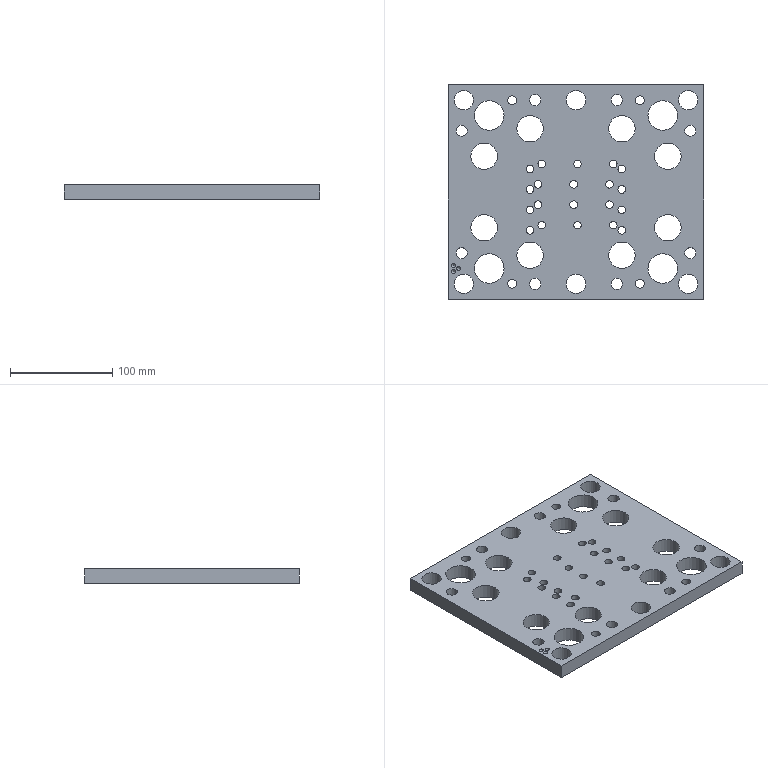Part | STEP file | 200 mesh_id2102 | 1 solid | 59 faces | box 250 x 210 x 14 mm | volume 588514 mm3 | cylinder 50 | plane 6 | cone 3 | commonest cylinder face diameters 7.5 x20 11 x8 26 x8 19 x6 8.5 x4 29 x4